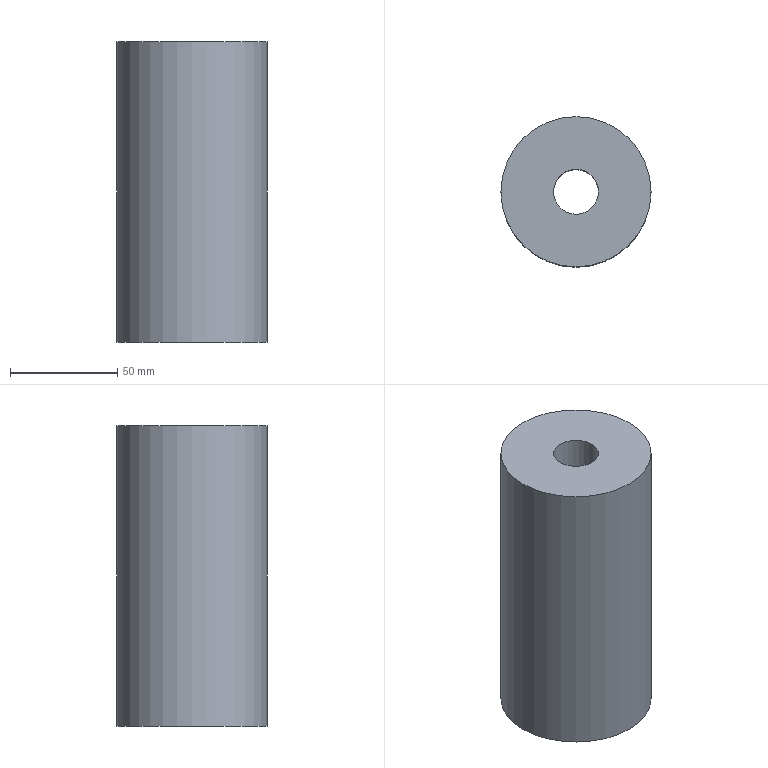Part | NX | features solid 2 | 1 solid | 4 faces | box 70 x 70 x 140 mm | volume 490293 mm3 | cylinder 2 | plane 2 | commonest cylinder face diameters 21 x1 70 x1
STEP:
#1=CARTESIAN_POINT('',(-1044.749,664.749,-105.));
#2=VERTEX_POINT('',#1);
#3=CARTESIAN_POINT('',(-1020.,640.,-105.));
#4=DIRECTION('',(0.,0.,1.));
#5=DIRECTION('',(-0.7071,0.7071,0.));
#6=AXIS2_PLACEMENT_3D('',#3,#4,#5);
#7=CIRCLE('',#6,35.);
#8=EDGE_CURVE('',#2,#2,#7,.T.);
#9=ORIENTED_EDGE('',*,*,#8,.T.);
#10=EDGE_LOOP('',(#9));
#11=FACE_BOUND('',#10,.T.);
#12=CARTESIAN_POINT('',(-1044.749,664.749,35.));
#13=VERTEX_POINT('',#12);
#14=CARTESIAN_POINT('',(-1020.,640.,35.));
#15=DIRECTION('',(0.,0.,1.));
#16=DIRECTION('',(-0.7071,0.7071,0.));
#17=AXIS2_PLACEMENT_3D('',#14,#15,#16);
#18=CIRCLE('',#17,35.);
#19=EDGE_CURVE('',#13,#13,#18,.T.);
#20=ORIENTED_EDGE('',*,*,#19,.F.);
#21=EDGE_LOOP('',(#20));
#22=FACE_BOUND('',#21,.T.);
#23=CARTESIAN_POINT('',(-1020.,640.,-105.));
#24=DIRECTION('',(0.,0.,-1.));
#25=DIRECTION('',(-0.7071,0.7071,0.));
#26=AXIS2_PLACEMENT_3D('',#23,#24,#25);
#27=CYLINDRICAL_SURFACE('',#26,35.);
#28=ADVANCED_FACE('',(#11,#22),#27,.T.);
#29=CARTESIAN_POINT('',(-1027.425,647.425,-105.));
#30=VERTEX_POINT('',#29);
#31=CARTESIAN_POINT('',(-1020.,640.,-105.));
#32=DIRECTION('',(0.,0.,1.));
#33=DIRECTION('',(-0.7071,0.7071,0.));
#34=AXIS2_PLACEMENT_3D('',#31,#32,#33);
#35=CIRCLE('',#34,10.5);
#36=EDGE_CURVE('',#30,#30,#35,.T.);
#37=ORIENTED_EDGE('',*,*,#36,.T.);
#38=EDGE_LOOP('',(#37));
#39=FACE_BOUND('',#38,.T.);
#40=ORIENTED_EDGE('',*,*,#8,.F.);
#41=EDGE_LOOP('',(#40));
#42=FACE_BOUND('',#41,.T.);
#43=CARTESIAN_POINT('',(-1044.749,615.251,-105.));
#44=DIRECTION('',(0.,0.,1.));
#45=DIRECTION('',(0.7071,-0.7071,0.));
#46=AXIS2_PLACEMENT_3D('',#43,#44,#45);
#47=PLANE('',#46);
#48=ADVANCED_FACE('',(#39,#42),#47,.F.);
#49=CARTESIAN_POINT('',(-1027.425,647.425,35.));
#50=VERTEX_POINT('',#49);
#51=CARTESIAN_POINT('',(-1020.,640.,35.));
#52=DIRECTION('',(0.,0.,1.));
#53=DIRECTION('',(-0.7071,0.7071,0.));
#54=AXIS2_PLACEMENT_3D('',#51,#52,#53);
#55=CIRCLE('',#54,10.5);
#56=EDGE_CURVE('',#50,#50,#55,.T.);
#57=ORIENTED_EDGE('',*,*,#56,.T.);
#58=EDGE_LOOP('',(#57));
#59=FACE_BOUND('',#58,.T.);
#60=ORIENTED_EDGE('',*,*,#36,.F.);
#61=EDGE_LOOP('',(#60));
#62=FACE_BOUND('',#61,.T.);
#63=CARTESIAN_POINT('',(-1020.,640.,-105.));
#64=DIRECTION('',(0.,0.,-1.));
#65=DIRECTION('',(-0.7071,0.7071,0.));
#66=AXIS2_PLACEMENT_3D('',#63,#64,#65);
#67=CYLINDRICAL_SURFACE('',#66,10.5);
#68=ADVANCED_FACE('',(#59,#62),#67,.F.);
#69=ORIENTED_EDGE('',*,*,#19,.T.);
#70=EDGE_LOOP('',(#69));
#71=FACE_BOUND('',#70,.T.);
#72=ORIENTED_EDGE('',*,*,#56,.F.);
#73=EDGE_LOOP('',(#72));
#74=FACE_BOUND('',#73,.T.);
#75=CARTESIAN_POINT('',(-1027.425,632.575,35.));
#76=DIRECTION('',(0.,0.,-1.));
#77=DIRECTION('',(-0.7071,0.7071,0.));
#78=AXIS2_PLACEMENT_3D('',#75,#76,#77);
#79=PLANE('',#78);
#80=ADVANCED_FACE('',(#71,#74),#79,.F.);
#81=CLOSED_SHELL('',(#28,#48,#68,#80));
#82=MANIFOLD_SOLID_BREP('',#81);
#83=(LENGTH_UNIT()NAMED_UNIT(*)SI_UNIT(.MILLI.,.METRE.));
#84=UNCERTAINTY_MEASURE_WITH_UNIT(LENGTH_MEASURE(0.00001),#83,'','');
#85=(NAMED_UNIT(*)PLANE_ANGLE_UNIT()SI_UNIT($,.RADIAN.));
#86=(NAMED_UNIT(*)SI_UNIT($,.STERADIAN.)SOLID_ANGLE_UNIT());
#87=(GEOMETRIC_REPRESENTATION_CONTEXT(3)GLOBAL_UNCERTAINTY_ASSIGNED_CONTEXT((#84))GLOBAL_UNIT_ASSIGNED_CONTEXT((#83,#85,#86))REPRESENTATION_CONTEXT('',''));
#88=ADVANCED_BREP_SHAPE_REPRESENTATION('',(#82),#87);